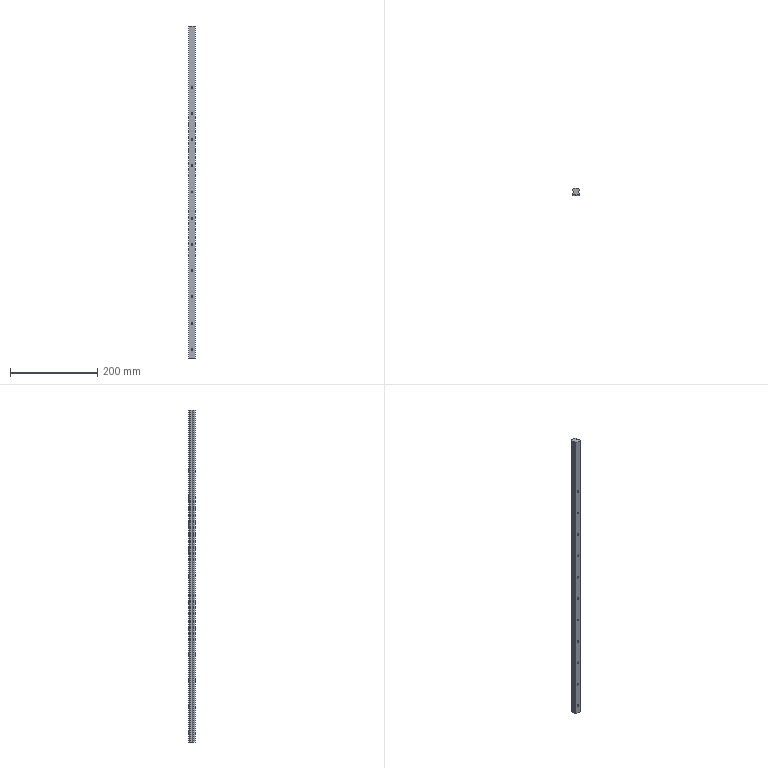Part | STEP file | Guide rail HGH15 (HGH15 rail) | 1 solid | 79 faces | box 15 x 15 x 760 mm | volume 145713 mm3 | cylinder 50 | plane 29 | commonest cylinder face diameters 4.5 x22 7.5 x22 0.8 x6